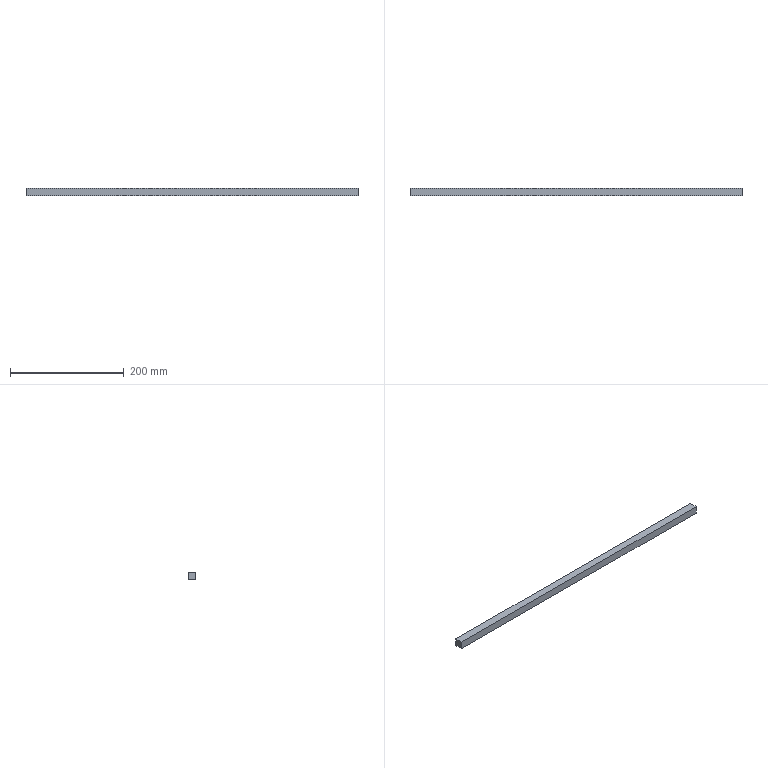Part | NX | features solid 2 | 1 solid | 6 faces | box 585 x 14 x 14 mm | volume 114660 mm3 | plane 6
STEP:
#1=CARTESIAN_POINT('',(300.,296.,-5.));
#2=VERTEX_POINT('',#1);
#3=CARTESIAN_POINT('',(-285.,296.,-5.));
#4=VERTEX_POINT('',#3);
#5=CARTESIAN_POINT('',(300.,296.,-5.));
#6=DIRECTION('',(-1.,0.,0.));
#7=VECTOR('',#6,1000.);
#8=LINE('',#5,#7);
#9=EDGE_CURVE('',#2,#4,#8,.T.);
#10=ORIENTED_EDGE('',*,*,#9,.F.);
#11=CARTESIAN_POINT('',(300.,296.,9.));
#12=VERTEX_POINT('',#11);
#13=CARTESIAN_POINT('',(300.,296.,9.));
#14=DIRECTION('',(0.,0.,-1.));
#15=VECTOR('',#14,1000.);
#16=LINE('',#13,#15);
#17=EDGE_CURVE('',#12,#2,#16,.T.);
#18=ORIENTED_EDGE('',*,*,#17,.F.);
#19=CARTESIAN_POINT('',(-285.,296.,9.));
#20=VERTEX_POINT('',#19);
#21=CARTESIAN_POINT('',(300.,296.,9.));
#22=DIRECTION('',(-1.,0.,0.));
#23=VECTOR('',#22,1000.);
#24=LINE('',#21,#23);
#25=EDGE_CURVE('',#12,#20,#24,.T.);
#26=ORIENTED_EDGE('',*,*,#25,.T.);
#27=CARTESIAN_POINT('',(-285.,296.,9.));
#28=DIRECTION('',(0.,0.,-1.));
#29=VECTOR('',#28,1000.);
#30=LINE('',#27,#29);
#31=EDGE_CURVE('',#20,#4,#30,.T.);
#32=ORIENTED_EDGE('',*,*,#31,.T.);
#33=EDGE_LOOP('',(#10,#18,#26,#32));
#34=FACE_BOUND('',#33,.T.);
#35=CARTESIAN_POINT('',(300.,296.,9.));
#36=DIRECTION('',(0.,-1.,0.));
#37=DIRECTION('',(0.,0.,-1.));
#38=AXIS2_PLACEMENT_3D('',#35,#36,#37);
#39=PLANE('',#38);
#40=ADVANCED_FACE('',(#34),#39,.T.);
#41=CARTESIAN_POINT('',(300.,310.,-5.));
#42=VERTEX_POINT('',#41);
#43=CARTESIAN_POINT('',(300.,335.,-5.));
#44=DIRECTION('',(0.,-1.,0.));
#45=VECTOR('',#44,1000.);
#46=LINE('',#43,#45);
#47=EDGE_CURVE('',#42,#2,#46,.T.);
#48=ORIENTED_EDGE('',*,*,#47,.F.);
#49=CARTESIAN_POINT('',(300.,310.,9.));
#50=VERTEX_POINT('',#49);
#51=CARTESIAN_POINT('',(300.,310.,9.));
#52=DIRECTION('',(0.,0.,-1.));
#53=VECTOR('',#52,1000.);
#54=LINE('',#51,#53);
#55=EDGE_CURVE('',#50,#42,#54,.T.);
#56=ORIENTED_EDGE('',*,*,#55,.F.);
#57=CARTESIAN_POINT('',(300.,335.,9.));
#58=DIRECTION('',(0.,-1.,0.));
#59=VECTOR('',#58,1000.);
#60=LINE('',#57,#59);
#61=EDGE_CURVE('',#50,#12,#60,.T.);
#62=ORIENTED_EDGE('',*,*,#61,.T.);
#63=ORIENTED_EDGE('',*,*,#17,.T.);
#64=EDGE_LOOP('',(#48,#56,#62,#63));
#65=FACE_BOUND('',#64,.T.);
#66=CARTESIAN_POINT('',(300.,335.,9.));
#67=DIRECTION('',(1.,0.,0.));
#68=DIRECTION('',(0.,0.,-1.));
#69=AXIS2_PLACEMENT_3D('',#66,#67,#68);
#70=PLANE('',#69);
#71=ADVANCED_FACE('',(#65),#70,.T.);
#72=CARTESIAN_POINT('',(-285.,310.,-5.));
#73=VERTEX_POINT('',#72);
#74=CARTESIAN_POINT('',(300.,310.,-5.));
#75=DIRECTION('',(-1.,0.,0.));
#76=VECTOR('',#75,1000.);
#77=LINE('',#74,#76);
#78=EDGE_CURVE('',#42,#73,#77,.T.);
#79=ORIENTED_EDGE('',*,*,#78,.T.);
#80=CARTESIAN_POINT('',(-285.,310.,9.));
#81=VERTEX_POINT('',#80);
#82=CARTESIAN_POINT('',(-285.,310.,9.));
#83=DIRECTION('',(0.,0.,-1.));
#84=VECTOR('',#83,1000.);
#85=LINE('',#82,#84);
#86=EDGE_CURVE('',#81,#73,#85,.T.);
#87=ORIENTED_EDGE('',*,*,#86,.F.);
#88=CARTESIAN_POINT('',(300.,310.,9.));
#89=DIRECTION('',(-1.,0.,0.));
#90=VECTOR('',#89,1000.);
#91=LINE('',#88,#90);
#92=EDGE_CURVE('',#50,#81,#91,.T.);
#93=ORIENTED_EDGE('',*,*,#92,.F.);
#94=ORIENTED_EDGE('',*,*,#55,.T.);
#95=EDGE_LOOP('',(#79,#87,#93,#94));
#96=FACE_BOUND('',#95,.T.);
#97=CARTESIAN_POINT('',(300.,310.,9.));
#98=DIRECTION('',(0.,-1.,0.));
#99=DIRECTION('',(0.,0.,-1.));
#100=AXIS2_PLACEMENT_3D('',#97,#98,#99);
#101=PLANE('',#100);
#102=ADVANCED_FACE('',(#96),#101,.F.);
#103=CARTESIAN_POINT('',(-285.,335.,-5.));
#104=DIRECTION('',(0.,-1.,0.));
#105=VECTOR('',#104,1000.);
#106=LINE('',#103,#105);
#107=EDGE_CURVE('',#73,#4,#106,.T.);
#108=ORIENTED_EDGE('',*,*,#107,.T.);
#109=ORIENTED_EDGE('',*,*,#31,.F.);
#110=CARTESIAN_POINT('',(-285.,335.,9.));
#111=DIRECTION('',(0.,-1.,0.));
#112=VECTOR('',#111,1000.);
#113=LINE('',#110,#112);
#114=EDGE_CURVE('',#81,#20,#113,.T.);
#115=ORIENTED_EDGE('',*,*,#114,.F.);
#116=ORIENTED_EDGE('',*,*,#86,.T.);
#117=EDGE_LOOP('',(#108,#109,#115,#116));
#118=FACE_BOUND('',#117,.T.);
#119=CARTESIAN_POINT('',(-285.,335.,9.));
#120=DIRECTION('',(1.,0.,0.));
#121=DIRECTION('',(0.,0.,-1.));
#122=AXIS2_PLACEMENT_3D('',#119,#120,#121);
#123=PLANE('',#122);
#124=ADVANCED_FACE('',(#118),#123,.F.);
#125=ORIENTED_EDGE('',*,*,#25,.F.);
#126=ORIENTED_EDGE('',*,*,#61,.F.);
#127=ORIENTED_EDGE('',*,*,#92,.T.);
#128=ORIENTED_EDGE('',*,*,#114,.T.);
#129=EDGE_LOOP('',(#125,#126,#127,#128));
#130=FACE_BOUND('',#129,.T.);
#131=CARTESIAN_POINT('',(153.75,319.,9.));
#132=DIRECTION('',(0.,0.,1.));
#133=DIRECTION('',(1.,0.,0.));
#134=AXIS2_PLACEMENT_3D('',#131,#132,#133);
#135=PLANE('',#134);
#136=ADVANCED_FACE('',(#130),#135,.T.);
#137=ORIENTED_EDGE('',*,*,#9,.T.);
#138=ORIENTED_EDGE('',*,*,#107,.F.);
#139=ORIENTED_EDGE('',*,*,#78,.F.);
#140=ORIENTED_EDGE('',*,*,#47,.T.);
#141=EDGE_LOOP('',(#137,#138,#139,#140));
#142=FACE_BOUND('',#141,.T.);
#143=CARTESIAN_POINT('',(153.75,319.,-5.));
#144=DIRECTION('',(0.,0.,1.));
#145=DIRECTION('',(1.,0.,0.));
#146=AXIS2_PLACEMENT_3D('',#143,#144,#145);
#147=PLANE('',#146);
#148=ADVANCED_FACE('',(#142),#147,.F.);
#149=CLOSED_SHELL('',(#40,#71,#102,#124,#136,#148));
#150=MANIFOLD_SOLID_BREP('',#149);
#151=(LENGTH_UNIT()NAMED_UNIT(*)SI_UNIT(.MILLI.,.METRE.));
#152=UNCERTAINTY_MEASURE_WITH_UNIT(LENGTH_MEASURE(0.00001),#151,'','');
#153=(NAMED_UNIT(*)PLANE_ANGLE_UNIT()SI_UNIT($,.RADIAN.));
#154=(NAMED_UNIT(*)SI_UNIT($,.STERADIAN.)SOLID_ANGLE_UNIT());
#155=(GEOMETRIC_REPRESENTATION_CONTEXT(3)GLOBAL_UNCERTAINTY_ASSIGNED_CONTEXT((#152))GLOBAL_UNIT_ASSIGNED_CONTEXT((#151,#153,#154))REPRESENTATION_CONTEXT('',''));
#156=ADVANCED_BREP_SHAPE_REPRESENTATION('',(#150),#155);